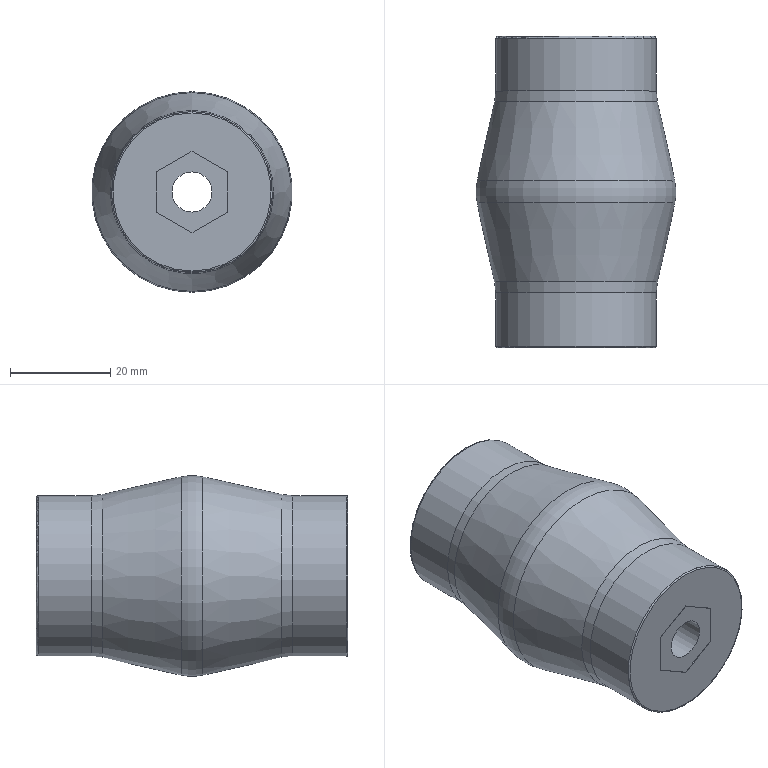Part | STEP file | PN_0016_default | 1 solid | 25 faces | box 40 x 62 x 40 mm | volume 28151 mm3 | plane 10 | torus 6 | cylinder 5 | cone 4 | commonest cylinder face diameters 24 x2 32 x2 8 x1